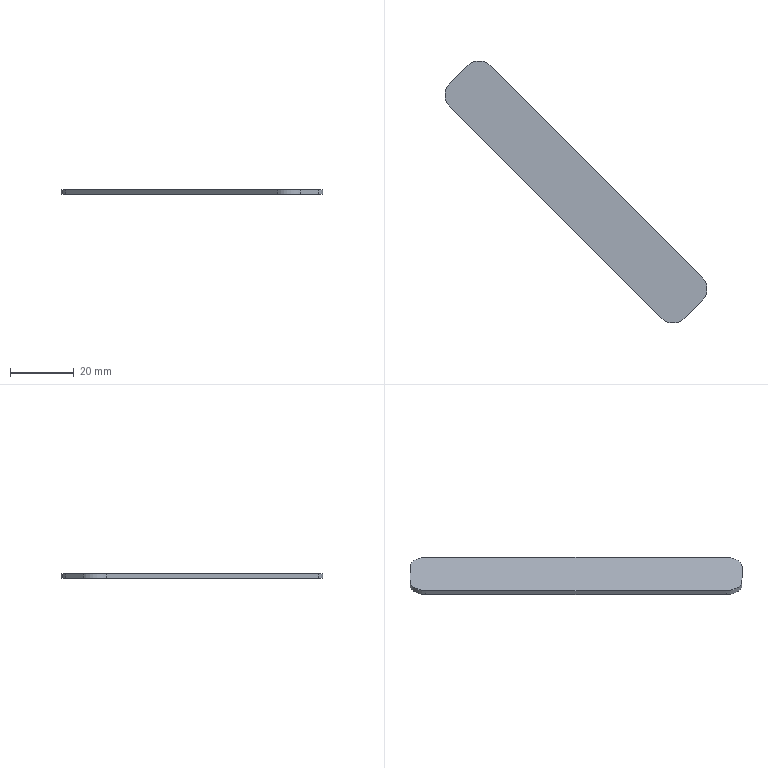Part | NX | features BREP 1 | 1 solid | 10 faces | box 82.125 x 82.125 x 1.5 mm | volume 2776 mm3 | plane 6 | cylinder 4 | commonest cylinder face diameters 10 x4
STEP:
#1=CARTESIAN_POINT('',(-3.536,144.169,0.));
#2=VERTEX_POINT('',#1);
#3=CARTESIAN_POINT('',(-9.192,138.512,0.));
#4=VERTEX_POINT('',#3);
#5=CARTESIAN_POINT('',(-3.536,144.169,0.));
#6=DIRECTION('',(-0.7071,-0.7071,0.));
#7=VECTOR('',#6,1000.);
#8=LINE('',#5,#7);
#9=EDGE_CURVE('',#2,#4,#8,.T.);
#10=ORIENTED_EDGE('',*,*,#9,.T.);
#11=CARTESIAN_POINT('',(-9.192,131.441,0.));
#12=VERTEX_POINT('',#11);
#13=CARTESIAN_POINT('',(-5.657,134.976,0.));
#14=DIRECTION('',(0.,0.,1.));
#15=DIRECTION('',(-0.7071,0.7071,0.));
#16=AXIS2_PLACEMENT_3D('',#13,#14,#15);
#17=CIRCLE('',#16,5.);
#18=EDGE_CURVE('',#4,#12,#17,.T.);
#19=ORIENTED_EDGE('',*,*,#18,.T.);
#20=CARTESIAN_POINT('',(57.276,64.973,0.));
#21=VERTEX_POINT('',#20);
#22=CARTESIAN_POINT('',(-9.192,131.441,0.));
#23=DIRECTION('',(0.7071,-0.7071,0.));
#24=VECTOR('',#23,1000.);
#25=LINE('',#22,#24);
#26=EDGE_CURVE('',#12,#21,#25,.T.);
#27=ORIENTED_EDGE('',*,*,#26,.T.);
#28=CARTESIAN_POINT('',(64.347,64.973,0.));
#29=VERTEX_POINT('',#28);
#30=CARTESIAN_POINT('',(60.811,68.508,0.));
#31=DIRECTION('',(0.,0.,1.));
#32=DIRECTION('',(-0.7071,-0.7071,0.));
#33=AXIS2_PLACEMENT_3D('',#30,#31,#32);
#34=CIRCLE('',#33,5.);
#35=EDGE_CURVE('',#21,#29,#34,.T.);
#36=ORIENTED_EDGE('',*,*,#35,.T.);
#37=CARTESIAN_POINT('',(70.004,70.629,0.));
#38=VERTEX_POINT('',#37);
#39=CARTESIAN_POINT('',(64.347,64.973,0.));
#40=DIRECTION('',(0.7071,0.7071,0.));
#41=VECTOR('',#40,1000.);
#42=LINE('',#39,#41);
#43=EDGE_CURVE('',#29,#38,#42,.T.);
#44=ORIENTED_EDGE('',*,*,#43,.T.);
#45=CARTESIAN_POINT('',(70.004,77.701,0.));
#46=VERTEX_POINT('',#45);
#47=CARTESIAN_POINT('',(66.468,74.165,0.));
#48=DIRECTION('',(0.,0.,1.));
#49=DIRECTION('',(0.7071,-0.7071,0.));
#50=AXIS2_PLACEMENT_3D('',#47,#48,#49);
#51=CIRCLE('',#50,5.);
#52=EDGE_CURVE('',#38,#46,#51,.T.);
#53=ORIENTED_EDGE('',*,*,#52,.T.);
#54=CARTESIAN_POINT('',(3.536,144.169,0.));
#55=VERTEX_POINT('',#54);
#56=CARTESIAN_POINT('',(70.004,77.701,0.));
#57=DIRECTION('',(-0.7071,0.7071,0.));
#58=VECTOR('',#57,1000.);
#59=LINE('',#56,#58);
#60=EDGE_CURVE('',#46,#55,#59,.T.);
#61=ORIENTED_EDGE('',*,*,#60,.T.);
#62=CARTESIAN_POINT('',(0.,140.633,0.));
#63=DIRECTION('',(0.,0.,1.));
#64=DIRECTION('',(0.7071,0.7071,0.));
#65=AXIS2_PLACEMENT_3D('',#62,#63,#64);
#66=CIRCLE('',#65,5.);
#67=EDGE_CURVE('',#55,#2,#66,.T.);
#68=ORIENTED_EDGE('',*,*,#67,.T.);
#69=EDGE_LOOP('',(#10,#19,#27,#36,#44,#53,#61,#68));
#70=FACE_BOUND('',#69,.T.);
#71=CARTESIAN_POINT('',(0.,0.,0.));
#72=DIRECTION('',(0.,0.,1.));
#73=DIRECTION('',(1.,0.,0.));
#74=AXIS2_PLACEMENT_3D('',#71,#72,#73);
#75=PLANE('',#74);
#76=ADVANCED_FACE('',(#70),#75,.T.);
#77=CARTESIAN_POINT('',(3.536,144.169,-1.5));
#78=VERTEX_POINT('',#77);
#79=CARTESIAN_POINT('',(3.536,144.169,-1.5));
#80=DIRECTION('',(0.,0.,1.));
#81=VECTOR('',#80,1000.);
#82=LINE('',#79,#81);
#83=EDGE_CURVE('',#78,#55,#82,.T.);
#84=ORIENTED_EDGE('',*,*,#83,.F.);
#85=CARTESIAN_POINT('',(-3.536,144.169,-1.5));
#86=VERTEX_POINT('',#85);
#87=CARTESIAN_POINT('',(0.,140.633,-1.5));
#88=DIRECTION('',(0.,0.,-1.));
#89=DIRECTION('',(-0.7071,0.7071,0.));
#90=AXIS2_PLACEMENT_3D('',#87,#88,#89);
#91=CIRCLE('',#90,5.);
#92=EDGE_CURVE('',#86,#78,#91,.T.);
#93=ORIENTED_EDGE('',*,*,#92,.F.);
#94=CARTESIAN_POINT('',(-3.536,144.169,-1.5));
#95=DIRECTION('',(0.,0.,1.));
#96=VECTOR('',#95,1000.);
#97=LINE('',#94,#96);
#98=EDGE_CURVE('',#86,#2,#97,.T.);
#99=ORIENTED_EDGE('',*,*,#98,.T.);
#100=ORIENTED_EDGE('',*,*,#67,.F.);
#101=EDGE_LOOP('',(#84,#93,#99,#100));
#102=FACE_BOUND('',#101,.T.);
#103=CARTESIAN_POINT('',(0.,140.633,-7.664));
#104=DIRECTION('',(0.,0.,1.));
#105=DIRECTION('',(0.7071,0.7071,0.));
#106=AXIS2_PLACEMENT_3D('',#103,#104,#105);
#107=CYLINDRICAL_SURFACE('',#106,5.);
#108=ADVANCED_FACE('',(#102),#107,.T.);
#109=CARTESIAN_POINT('',(-9.192,138.512,-1.5));
#110=VERTEX_POINT('',#109);
#111=CARTESIAN_POINT('',(-3.536,144.169,-1.5));
#112=DIRECTION('',(-0.7071,-0.7071,0.));
#113=VECTOR('',#112,1000.);
#114=LINE('',#111,#113);
#115=EDGE_CURVE('',#86,#110,#114,.T.);
#116=ORIENTED_EDGE('',*,*,#115,.T.);
#117=CARTESIAN_POINT('',(-9.192,138.512,-1.5));
#118=DIRECTION('',(0.,0.,1.));
#119=VECTOR('',#118,1000.);
#120=LINE('',#117,#119);
#121=EDGE_CURVE('',#110,#4,#120,.T.);
#122=ORIENTED_EDGE('',*,*,#121,.T.);
#123=ORIENTED_EDGE('',*,*,#9,.F.);
#124=ORIENTED_EDGE('',*,*,#98,.F.);
#125=EDGE_LOOP('',(#116,#122,#123,#124));
#126=FACE_BOUND('',#125,.T.);
#127=CARTESIAN_POINT('',(-6.364,141.34,-0.75));
#128=DIRECTION('',(-0.7071,0.7071,0.));
#129=DIRECTION('',(0.,0.,1.));
#130=AXIS2_PLACEMENT_3D('',#127,#128,#129);
#131=PLANE('',#130);
#132=ADVANCED_FACE('',(#126),#131,.T.);
#133=ORIENTED_EDGE('',*,*,#121,.F.);
#134=CARTESIAN_POINT('',(-9.192,131.441,-1.5));
#135=VERTEX_POINT('',#134);
#136=CARTESIAN_POINT('',(-5.657,134.976,-1.5));
#137=DIRECTION('',(0.,0.,-1.));
#138=DIRECTION('',(-0.7071,-0.7071,0.));
#139=AXIS2_PLACEMENT_3D('',#136,#137,#138);
#140=CIRCLE('',#139,5.);
#141=EDGE_CURVE('',#135,#110,#140,.T.);
#142=ORIENTED_EDGE('',*,*,#141,.F.);
#143=CARTESIAN_POINT('',(-9.192,131.441,-1.5));
#144=DIRECTION('',(0.,0.,1.));
#145=VECTOR('',#144,1000.);
#146=LINE('',#143,#145);
#147=EDGE_CURVE('',#135,#12,#146,.T.);
#148=ORIENTED_EDGE('',*,*,#147,.T.);
#149=ORIENTED_EDGE('',*,*,#18,.F.);
#150=EDGE_LOOP('',(#133,#142,#148,#149));
#151=FACE_BOUND('',#150,.T.);
#152=CARTESIAN_POINT('',(-5.657,134.976,-7.664));
#153=DIRECTION('',(0.,0.,1.));
#154=DIRECTION('',(-0.7071,0.7071,0.));
#155=AXIS2_PLACEMENT_3D('',#152,#153,#154);
#156=CYLINDRICAL_SURFACE('',#155,5.);
#157=ADVANCED_FACE('',(#151),#156,.T.);
#158=CARTESIAN_POINT('',(57.276,64.973,-1.5));
#159=VERTEX_POINT('',#158);
#160=CARTESIAN_POINT('',(-9.192,131.441,-1.5));
#161=DIRECTION('',(0.7071,-0.7071,0.));
#162=VECTOR('',#161,1000.);
#163=LINE('',#160,#162);
#164=EDGE_CURVE('',#135,#159,#163,.T.);
#165=ORIENTED_EDGE('',*,*,#164,.T.);
#166=CARTESIAN_POINT('',(57.276,64.973,-1.5));
#167=DIRECTION('',(0.,0.,1.));
#168=VECTOR('',#167,1000.);
#169=LINE('',#166,#168);
#170=EDGE_CURVE('',#159,#21,#169,.T.);
#171=ORIENTED_EDGE('',*,*,#170,.T.);
#172=ORIENTED_EDGE('',*,*,#26,.F.);
#173=ORIENTED_EDGE('',*,*,#147,.F.);
#174=EDGE_LOOP('',(#165,#171,#172,#173));
#175=FACE_BOUND('',#174,.T.);
#176=CARTESIAN_POINT('',(24.042,98.207,-0.75));
#177=DIRECTION('',(-0.7071,-0.7071,0.));
#178=DIRECTION('',(-0.7071,0.7071,0.));
#179=AXIS2_PLACEMENT_3D('',#176,#177,#178);
#180=PLANE('',#179);
#181=ADVANCED_FACE('',(#175),#180,.T.);
#182=ORIENTED_EDGE('',*,*,#170,.F.);
#183=CARTESIAN_POINT('',(64.347,64.973,-1.5));
#184=VERTEX_POINT('',#183);
#185=CARTESIAN_POINT('',(60.811,68.508,-1.5));
#186=DIRECTION('',(0.,0.,-1.));
#187=DIRECTION('',(0.7071,-0.7071,0.));
#188=AXIS2_PLACEMENT_3D('',#185,#186,#187);
#189=CIRCLE('',#188,5.);
#190=EDGE_CURVE('',#184,#159,#189,.T.);
#191=ORIENTED_EDGE('',*,*,#190,.F.);
#192=CARTESIAN_POINT('',(64.347,64.973,-1.5));
#193=DIRECTION('',(0.,0.,1.));
#194=VECTOR('',#193,1000.);
#195=LINE('',#192,#194);
#196=EDGE_CURVE('',#184,#29,#195,.T.);
#197=ORIENTED_EDGE('',*,*,#196,.T.);
#198=ORIENTED_EDGE('',*,*,#35,.F.);
#199=EDGE_LOOP('',(#182,#191,#197,#198));
#200=FACE_BOUND('',#199,.T.);
#201=CARTESIAN_POINT('',(60.811,68.508,-7.664));
#202=DIRECTION('',(0.,0.,1.));
#203=DIRECTION('',(-0.7071,-0.7071,0.));
#204=AXIS2_PLACEMENT_3D('',#201,#202,#203);
#205=CYLINDRICAL_SURFACE('',#204,5.);
#206=ADVANCED_FACE('',(#200),#205,.T.);
#207=CARTESIAN_POINT('',(70.004,70.629,-1.5));
#208=VERTEX_POINT('',#207);
#209=CARTESIAN_POINT('',(64.347,64.973,-1.5));
#210=DIRECTION('',(0.7071,0.7071,0.));
#211=VECTOR('',#210,1000.);
#212=LINE('',#209,#211);
#213=EDGE_CURVE('',#184,#208,#212,.T.);
#214=ORIENTED_EDGE('',*,*,#213,.T.);
#215=CARTESIAN_POINT('',(70.004,70.629,-1.5));
#216=DIRECTION('',(0.,0.,1.));
#217=VECTOR('',#216,1000.);
#218=LINE('',#215,#217);
#219=EDGE_CURVE('',#208,#38,#218,.T.);
#220=ORIENTED_EDGE('',*,*,#219,.T.);
#221=ORIENTED_EDGE('',*,*,#43,.F.);
#222=ORIENTED_EDGE('',*,*,#196,.F.);
#223=EDGE_LOOP('',(#214,#220,#221,#222));
#224=FACE_BOUND('',#223,.T.);
#225=CARTESIAN_POINT('',(67.175,67.801,-0.75));
#226=DIRECTION('',(0.7071,-0.7071,0.));
#227=DIRECTION('',(0.,0.,-1.));
#228=AXIS2_PLACEMENT_3D('',#225,#226,#227);
#229=PLANE('',#228);
#230=ADVANCED_FACE('',(#224),#229,.T.);
#231=ORIENTED_EDGE('',*,*,#219,.F.);
#232=CARTESIAN_POINT('',(70.004,77.701,-1.5));
#233=VERTEX_POINT('',#232);
#234=CARTESIAN_POINT('',(66.468,74.165,-1.5));
#235=DIRECTION('',(0.,0.,-1.));
#236=DIRECTION('',(0.7071,0.7071,0.));
#237=AXIS2_PLACEMENT_3D('',#234,#235,#236);
#238=CIRCLE('',#237,5.);
#239=EDGE_CURVE('',#233,#208,#238,.T.);
#240=ORIENTED_EDGE('',*,*,#239,.F.);
#241=CARTESIAN_POINT('',(70.004,77.701,-1.5));
#242=DIRECTION('',(0.,0.,1.));
#243=VECTOR('',#242,1000.);
#244=LINE('',#241,#243);
#245=EDGE_CURVE('',#233,#46,#244,.T.);
#246=ORIENTED_EDGE('',*,*,#245,.T.);
#247=ORIENTED_EDGE('',*,*,#52,.F.);
#248=EDGE_LOOP('',(#231,#240,#246,#247));
#249=FACE_BOUND('',#248,.T.);
#250=CARTESIAN_POINT('',(66.468,74.165,-7.664));
#251=DIRECTION('',(0.,0.,1.));
#252=DIRECTION('',(0.7071,-0.7071,0.));
#253=AXIS2_PLACEMENT_3D('',#250,#251,#252);
#254=CYLINDRICAL_SURFACE('',#253,5.);
#255=ADVANCED_FACE('',(#249),#254,.T.);
#256=ORIENTED_EDGE('',*,*,#60,.F.);
#257=ORIENTED_EDGE('',*,*,#245,.F.);
#258=CARTESIAN_POINT('',(70.004,77.701,-1.5));
#259=DIRECTION('',(-0.7071,0.7071,0.));
#260=VECTOR('',#259,1000.);
#261=LINE('',#258,#260);
#262=EDGE_CURVE('',#233,#78,#261,.T.);
#263=ORIENTED_EDGE('',*,*,#262,.T.);
#264=ORIENTED_EDGE('',*,*,#83,.T.);
#265=EDGE_LOOP('',(#256,#257,#263,#264));
#266=FACE_BOUND('',#265,.T.);
#267=CARTESIAN_POINT('',(36.77,110.935,-0.75));
#268=DIRECTION('',(0.7071,0.7071,0.));
#269=DIRECTION('',(0.,0.,-1.));
#270=AXIS2_PLACEMENT_3D('',#267,#268,#269);
#271=PLANE('',#270);
#272=ADVANCED_FACE('',(#266),#271,.T.);
#273=ORIENTED_EDGE('',*,*,#262,.F.);
#274=ORIENTED_EDGE('',*,*,#239,.T.);
#275=ORIENTED_EDGE('',*,*,#213,.F.);
#276=ORIENTED_EDGE('',*,*,#190,.T.);
#277=ORIENTED_EDGE('',*,*,#164,.F.);
#278=ORIENTED_EDGE('',*,*,#141,.T.);
#279=ORIENTED_EDGE('',*,*,#115,.F.);
#280=ORIENTED_EDGE('',*,*,#92,.T.);
#281=EDGE_LOOP('',(#273,#274,#275,#276,#277,#278,#279,#280));
#282=FACE_BOUND('',#281,.T.);
#283=CARTESIAN_POINT('',(0.,0.,-1.5));
#284=DIRECTION('',(0.,0.,1.));
#285=DIRECTION('',(1.,0.,0.));
#286=AXIS2_PLACEMENT_3D('',#283,#284,#285);
#287=PLANE('',#286);
#288=ADVANCED_FACE('',(#282),#287,.F.);
#289=CLOSED_SHELL('',(#76,#108,#132,#157,#181,#206,#230,#255,#272,#288));
#290=MANIFOLD_SOLID_BREP('',#289);
#291=(LENGTH_UNIT()NAMED_UNIT(*)SI_UNIT(.MILLI.,.METRE.));
#292=UNCERTAINTY_MEASURE_WITH_UNIT(LENGTH_MEASURE(0.00001),#291,'','');
#293=(NAMED_UNIT(*)PLANE_ANGLE_UNIT()SI_UNIT($,.RADIAN.));
#294=(NAMED_UNIT(*)SI_UNIT($,.STERADIAN.)SOLID_ANGLE_UNIT());
#295=(GEOMETRIC_REPRESENTATION_CONTEXT(3)GLOBAL_UNCERTAINTY_ASSIGNED_CONTEXT((#292))GLOBAL_UNIT_ASSIGNED_CONTEXT((#291,#293,#294))REPRESENTATION_CONTEXT('',''));
#296=ADVANCED_BREP_SHAPE_REPRESENTATION('',(#290),#295);